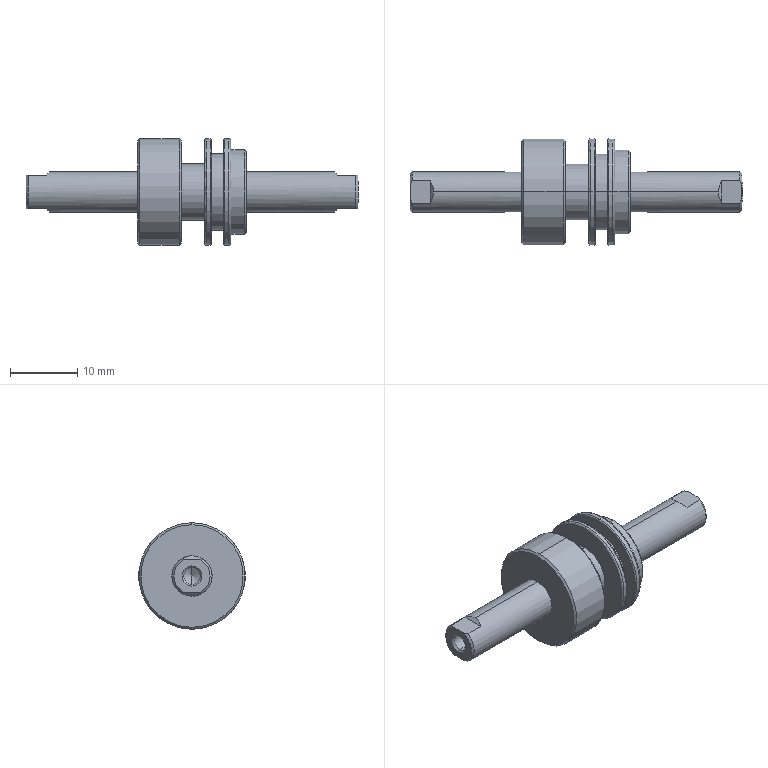Part | SolidWorks | features BaseBody 1 | 1 solid | 63 faces | box 49.5 x 15.9 x 15.9 mm | volume 3218 mm3 | cylinder 20 | cone 18 | plane 17 | spline 8 | commonest cylinder face diameters 15.9 x6 2.459 x4 6 x4 8.4 x2 11.4 x2 12.6 x2